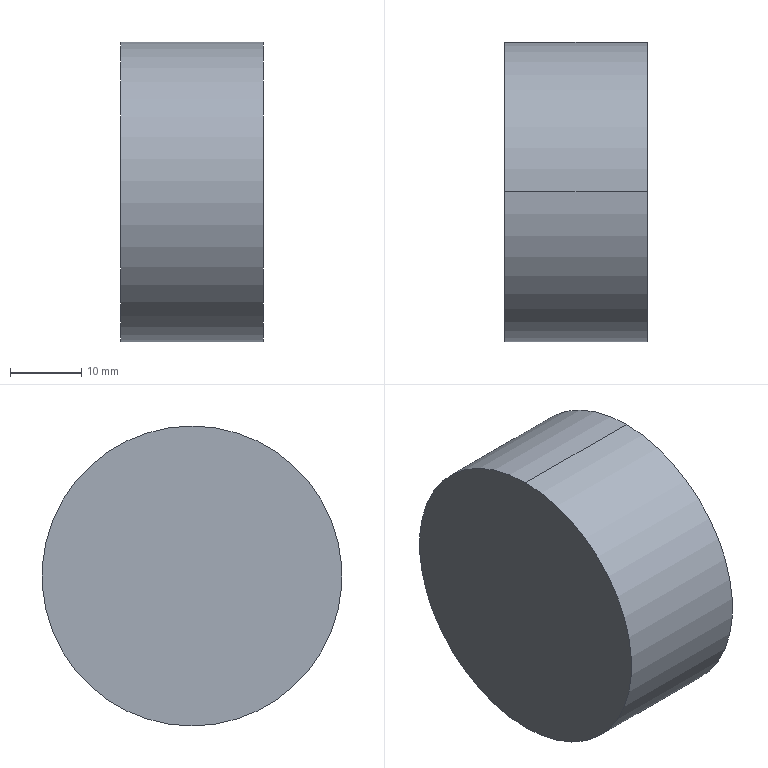Part | SolidWorks | features BaseBody 1 | 1 solid | 4 faces | box 20 x 42 x 42 mm | volume 27709 mm3 | cylinder 2 | plane 2 | commonest cylinder face diameters 42 x2
STEP:
#1=CARTESIAN_POINT('',(-60.,0.,-21.));
#2=VERTEX_POINT('',#1);
#3=CARTESIAN_POINT('',(-60.,0.,21.));
#4=VERTEX_POINT('',#3);
#5=CARTESIAN_POINT('',(-60.,0.,0.));
#6=DIRECTION('',(1.,0.,0.));
#7=DIRECTION('',(0.,0.,-1.));
#8=AXIS2_PLACEMENT_3D('',#5,#6,#7);
#9=CIRCLE('',#8,21.);
#10=EDGE_CURVE('',#2,#4,#9,.T.);
#11=ORIENTED_EDGE('',*,*,#10,.T.);
#12=CARTESIAN_POINT('',(-40.,0.,21.));
#13=VERTEX_POINT('',#12);
#14=CARTESIAN_POINT('',(-60.,0.,21.));
#15=DIRECTION('',(1.,0.,0.));
#16=VECTOR('',#15,1000.);
#17=LINE('',#14,#16);
#18=EDGE_CURVE('',#4,#13,#17,.T.);
#19=ORIENTED_EDGE('',*,*,#18,.T.);
#20=CARTESIAN_POINT('',(-40.,0.,-21.));
#21=VERTEX_POINT('',#20);
#22=CARTESIAN_POINT('',(-40.,0.,0.));
#23=DIRECTION('',(-1.,0.,0.));
#24=DIRECTION('',(0.,0.,-1.));
#25=AXIS2_PLACEMENT_3D('',#22,#23,#24);
#26=CIRCLE('',#25,21.);
#27=EDGE_CURVE('',#13,#21,#26,.T.);
#28=ORIENTED_EDGE('',*,*,#27,.T.);
#29=CARTESIAN_POINT('',(-60.,0.,-21.));
#30=DIRECTION('',(1.,0.,0.));
#31=VECTOR('',#30,1000.);
#32=LINE('',#29,#31);
#33=EDGE_CURVE('',#2,#21,#32,.T.);
#34=ORIENTED_EDGE('',*,*,#33,.F.);
#35=EDGE_LOOP('',(#11,#19,#28,#34));
#36=FACE_OUTER_BOUND('',#35,.T.);
#37=CARTESIAN_POINT('',(-60.,0.,0.));
#38=DIRECTION('',(1.,0.,0.));
#39=DIRECTION('',(0.,0.,-1.));
#40=AXIS2_PLACEMENT_3D('',#37,#38,#39);
#41=CYLINDRICAL_SURFACE('',#40,21.);
#42=ADVANCED_FACE('',(#36),#41,.T.);
#43=ORIENTED_EDGE('',*,*,#18,.F.);
#44=CARTESIAN_POINT('',(-60.,0.,0.));
#45=DIRECTION('',(1.,0.,0.));
#46=DIRECTION('',(0.,0.,-1.));
#47=AXIS2_PLACEMENT_3D('',#44,#45,#46);
#48=CIRCLE('',#47,21.);
#49=EDGE_CURVE('',#4,#2,#48,.T.);
#50=ORIENTED_EDGE('',*,*,#49,.T.);
#51=ORIENTED_EDGE('',*,*,#33,.T.);
#52=CARTESIAN_POINT('',(-40.,0.,0.));
#53=DIRECTION('',(-1.,0.,0.));
#54=DIRECTION('',(0.,0.,-1.));
#55=AXIS2_PLACEMENT_3D('',#52,#53,#54);
#56=CIRCLE('',#55,21.);
#57=EDGE_CURVE('',#21,#13,#56,.T.);
#58=ORIENTED_EDGE('',*,*,#57,.T.);
#59=EDGE_LOOP('',(#43,#50,#51,#58));
#60=FACE_OUTER_BOUND('',#59,.T.);
#61=CARTESIAN_POINT('',(-60.,0.,0.));
#62=DIRECTION('',(1.,0.,0.));
#63=DIRECTION('',(0.,0.,-1.));
#64=AXIS2_PLACEMENT_3D('',#61,#62,#63);
#65=CYLINDRICAL_SURFACE('',#64,21.);
#66=ADVANCED_FACE('',(#60),#65,.T.);
#67=ORIENTED_EDGE('',*,*,#10,.F.);
#68=ORIENTED_EDGE('',*,*,#49,.F.);
#69=EDGE_LOOP('',(#67,#68));
#70=FACE_OUTER_BOUND('',#69,.T.);
#71=CARTESIAN_POINT('',(-60.,0.,0.));
#72=DIRECTION('',(1.,0.,0.));
#73=DIRECTION('',(0.,0.,-1.));
#74=AXIS2_PLACEMENT_3D('',#71,#72,#73);
#75=PLANE('',#74);
#76=ADVANCED_FACE('',(#70),#75,.F.);
#77=ORIENTED_EDGE('',*,*,#57,.F.);
#78=ORIENTED_EDGE('',*,*,#27,.F.);
#79=EDGE_LOOP('',(#77,#78));
#80=FACE_OUTER_BOUND('',#79,.T.);
#81=CARTESIAN_POINT('',(-40.,0.,0.));
#82=DIRECTION('',(1.,0.,0.));
#83=DIRECTION('',(0.,0.,-1.));
#84=AXIS2_PLACEMENT_3D('',#81,#82,#83);
#85=PLANE('',#84);
#86=ADVANCED_FACE('',(#80),#85,.T.);
#87=CLOSED_SHELL('',(#42,#66,#76,#86));
#88=MANIFOLD_SOLID_BREP('',#87);
#89=CARTESIAN_POINT('',(0.,0.,0.));
#90=DIRECTION('',(0.,0.,1.));
#91=DIRECTION('',(1.,0.,0.));
#92=AXIS2_PLACEMENT_3D('',#89,#90,#91);
#93=(LENGTH_UNIT()NAMED_UNIT(*)SI_UNIT(.MILLI.,.METRE.));
#94=UNCERTAINTY_MEASURE_WITH_UNIT(LENGTH_MEASURE(0.00001),#93,'','');
#95=(NAMED_UNIT(*)PLANE_ANGLE_UNIT()SI_UNIT($,.RADIAN.));
#96=(NAMED_UNIT(*)SI_UNIT($,.STERADIAN.)SOLID_ANGLE_UNIT());
#97=(GEOMETRIC_REPRESENTATION_CONTEXT(3)GLOBAL_UNCERTAINTY_ASSIGNED_CONTEXT((#94))GLOBAL_UNIT_ASSIGNED_CONTEXT((#93,#95,#96))REPRESENTATION_CONTEXT('',''));
#98=ADVANCED_BREP_SHAPE_REPRESENTATION('',(#88,#92),#97);